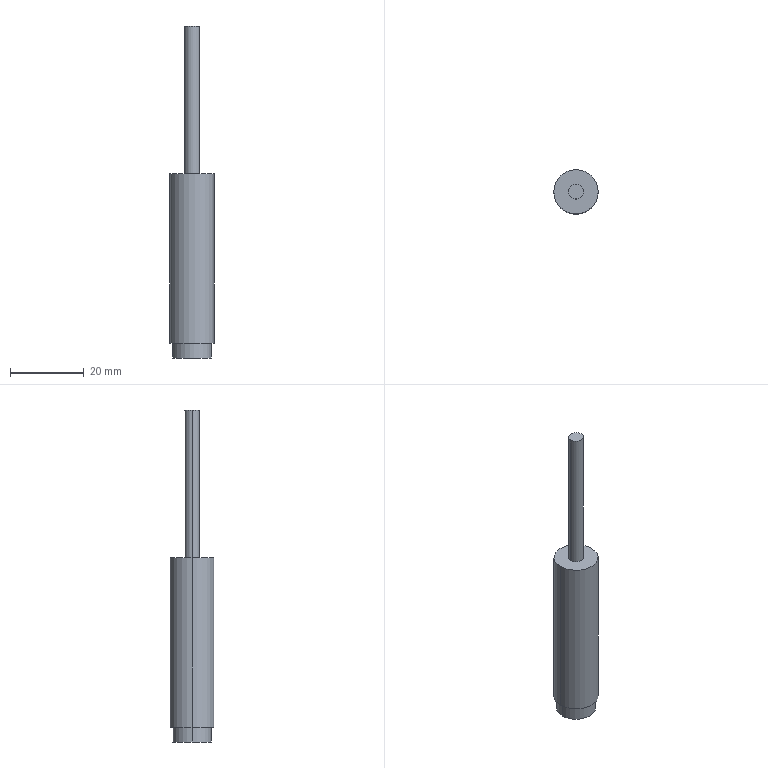Part | STEP file | PN_0035 (M12-4 proximity switch) | 1 solid | 10 faces | box 12 x 12 x 90 mm | volume 6055 mm3 | cylinder 6 | plane 4 | commonest cylinder face diameters 4 x2 10.55 x2 12 x2
STEP:
#1=CARTESIAN_POINT('',(0.,0.,0.));
#2=DIRECTION('',(0.,0.,1.));
#3=DIRECTION('',(1.,0.,0.));
#4=AXIS2_PLACEMENT_3D('',#1,#2,#3);
#5=CARTESIAN_POINT('',(2.,0.,90.));
#6=VERTEX_POINT('',#5);
#7=CARTESIAN_POINT('',(-2.,0.,90.));
#8=VERTEX_POINT('',#7);
#9=CARTESIAN_POINT('',(0.,0.,90.));
#10=DIRECTION('',(0.,0.,1.));
#11=DIRECTION('',(1.,0.,0.));
#12=AXIS2_PLACEMENT_3D('',#9,#10,#11);
#13=CIRCLE('',#12,2.);
#14=CARTESIAN_POINT('',(0.,0.,90.));
#15=DIRECTION('',(0.,0.,-1.));
#16=DIRECTION('',(-1.,0.,0.));
#17=AXIS2_PLACEMENT_3D('',#14,#15,#16);
#18=CYLINDRICAL_SURFACE('',#17,2.);
#19=CARTESIAN_POINT('',(3.142,0.));
#20=DIRECTION('',(-1.,0.));
#21=VECTOR('',#20,1.);
#22=LINE('',#19,#21);
#23=(GEOMETRIC_REPRESENTATION_CONTEXT(2)PARAMETRIC_REPRESENTATION_CONTEXT()REPRESENTATION_CONTEXT('',''));
#24=DEFINITIONAL_REPRESENTATION('',(#22),#23);
#25=PCURVE('',#18,#24);
#26=CARTESIAN_POINT('',(0.,0.,90.));
#27=DIRECTION('',(0.,0.,1.));
#28=DIRECTION('',(1.,0.,0.));
#29=AXIS2_PLACEMENT_3D('',#26,#27,#28);
#30=PLANE('',#29);
#31=CARTESIAN_POINT('',(0.,0.));
#32=DIRECTION('',(1.,0.));
#33=AXIS2_PLACEMENT_2D('',#31,#32);
#34=CIRCLE('',#33,2.);
#35=(GEOMETRIC_REPRESENTATION_CONTEXT(2)PARAMETRIC_REPRESENTATION_CONTEXT()REPRESENTATION_CONTEXT('',''));
#36=DEFINITIONAL_REPRESENTATION('',(#34),#35);
#37=PCURVE('',#30,#36);
#38=SURFACE_CURVE('',#13,(#25,#37),.PCURVE_S1.);
#39=EDGE_CURVE('',#6,#8,#38,.T.);
#40=ORIENTED_EDGE('',*,*,#39,.F.);
#41=CARTESIAN_POINT('',(2.,0.,50.));
#42=VERTEX_POINT('',#41);
#43=CARTESIAN_POINT('',(2.,0.,90.));
#44=DIRECTION('',(0.,0.,-1.));
#45=VECTOR('',#44,1.);
#46=LINE('',#43,#45);
#47=CARTESIAN_POINT('',(3.142,0.));
#48=DIRECTION('',(0.,1.));
#49=VECTOR('',#48,1.);
#50=LINE('',#47,#49);
#51=(GEOMETRIC_REPRESENTATION_CONTEXT(2)PARAMETRIC_REPRESENTATION_CONTEXT()REPRESENTATION_CONTEXT('',''));
#52=DEFINITIONAL_REPRESENTATION('',(#50),#51);
#53=PCURVE('',#18,#52);
#54=CARTESIAN_POINT('',(0.,0.,90.));
#55=DIRECTION('',(0.,0.,-1.));
#56=DIRECTION('',(-1.,0.,0.));
#57=AXIS2_PLACEMENT_3D('',#54,#55,#56);
#58=CYLINDRICAL_SURFACE('',#57,2.);
#59=CARTESIAN_POINT('',(3.142,0.));
#60=DIRECTION('',(0.,1.));
#61=VECTOR('',#60,1.);
#62=LINE('',#59,#61);
#63=(GEOMETRIC_REPRESENTATION_CONTEXT(2)PARAMETRIC_REPRESENTATION_CONTEXT()REPRESENTATION_CONTEXT('',''));
#64=DEFINITIONAL_REPRESENTATION('',(#62),#63);
#65=PCURVE('',#58,#64);
#66=SURFACE_CURVE('',#46,(#53,#65),.PCURVE_S1.);
#67=EDGE_CURVE('',#6,#42,#66,.T.);
#68=ORIENTED_EDGE('',*,*,#67,.T.);
#69=CARTESIAN_POINT('',(-2.,0.,50.));
#70=VERTEX_POINT('',#69);
#71=CARTESIAN_POINT('',(0.,0.,50.));
#72=DIRECTION('',(0.,0.,1.));
#73=DIRECTION('',(1.,0.,0.));
#74=AXIS2_PLACEMENT_3D('',#71,#72,#73);
#75=CIRCLE('',#74,2.);
#76=CARTESIAN_POINT('',(3.142,40.));
#77=DIRECTION('',(-1.,0.));
#78=VECTOR('',#77,1.);
#79=LINE('',#76,#78);
#80=(GEOMETRIC_REPRESENTATION_CONTEXT(2)PARAMETRIC_REPRESENTATION_CONTEXT()REPRESENTATION_CONTEXT('',''));
#81=DEFINITIONAL_REPRESENTATION('',(#79),#80);
#82=PCURVE('',#18,#81);
#83=CARTESIAN_POINT('',(0.,0.,50.));
#84=DIRECTION('',(0.,0.,1.));
#85=DIRECTION('',(1.,0.,0.));
#86=AXIS2_PLACEMENT_3D('',#83,#84,#85);
#87=PLANE('',#86);
#88=CARTESIAN_POINT('',(0.,0.));
#89=DIRECTION('',(1.,0.));
#90=AXIS2_PLACEMENT_2D('',#88,#89);
#91=CIRCLE('',#90,2.);
#92=(GEOMETRIC_REPRESENTATION_CONTEXT(2)PARAMETRIC_REPRESENTATION_CONTEXT()REPRESENTATION_CONTEXT('',''));
#93=DEFINITIONAL_REPRESENTATION('',(#91),#92);
#94=PCURVE('',#87,#93);
#95=SURFACE_CURVE('',#75,(#82,#94),.PCURVE_S1.);
#96=EDGE_CURVE('',#42,#70,#95,.T.);
#97=ORIENTED_EDGE('',*,*,#96,.T.);
#98=CARTESIAN_POINT('',(-2.,0.,90.));
#99=DIRECTION('',(0.,0.,-1.));
#100=VECTOR('',#99,1.);
#101=LINE('',#98,#100);
#102=CARTESIAN_POINT('',(0.,0.));
#103=DIRECTION('',(0.,1.));
#104=VECTOR('',#103,1.);
#105=LINE('',#102,#104);
#106=(GEOMETRIC_REPRESENTATION_CONTEXT(2)PARAMETRIC_REPRESENTATION_CONTEXT()REPRESENTATION_CONTEXT('',''));
#107=DEFINITIONAL_REPRESENTATION('',(#105),#106);
#108=PCURVE('',#18,#107);
#109=CARTESIAN_POINT('',(6.283,0.));
#110=DIRECTION('',(0.,1.));
#111=VECTOR('',#110,1.);
#112=LINE('',#109,#111);
#113=(GEOMETRIC_REPRESENTATION_CONTEXT(2)PARAMETRIC_REPRESENTATION_CONTEXT()REPRESENTATION_CONTEXT('',''));
#114=DEFINITIONAL_REPRESENTATION('',(#112),#113);
#115=PCURVE('',#58,#114);
#116=SURFACE_CURVE('',#101,(#108,#115),.PCURVE_S1.);
#117=EDGE_CURVE('',#8,#70,#116,.T.);
#118=ORIENTED_EDGE('',*,*,#117,.F.);
#119=EDGE_LOOP('',(#40,#68,#97,#118));
#120=FACE_BOUND('',#119,.T.);
#121=ADVANCED_FACE('',(#120),#18,.T.);
#122=CARTESIAN_POINT('',(6.,0.,50.));
#123=VERTEX_POINT('',#122);
#124=CARTESIAN_POINT('',(-6.,0.,50.));
#125=VERTEX_POINT('',#124);
#126=CARTESIAN_POINT('',(0.,0.,50.));
#127=DIRECTION('',(0.,0.,1.));
#128=DIRECTION('',(1.,0.,0.));
#129=AXIS2_PLACEMENT_3D('',#126,#127,#128);
#130=CIRCLE('',#129,6.);
#131=CARTESIAN_POINT('',(0.,0.,50.));
#132=DIRECTION('',(0.,0.,-1.));
#133=DIRECTION('',(-1.,0.,0.));
#134=AXIS2_PLACEMENT_3D('',#131,#132,#133);
#135=CYLINDRICAL_SURFACE('',#134,6.);
#136=CARTESIAN_POINT('',(3.142,0.));
#137=DIRECTION('',(-1.,0.));
#138=VECTOR('',#137,1.);
#139=LINE('',#136,#138);
#140=(GEOMETRIC_REPRESENTATION_CONTEXT(2)PARAMETRIC_REPRESENTATION_CONTEXT()REPRESENTATION_CONTEXT('',''));
#141=DEFINITIONAL_REPRESENTATION('',(#139),#140);
#142=PCURVE('',#135,#141);
#143=CARTESIAN_POINT('',(0.,0.));
#144=DIRECTION('',(1.,0.));
#145=AXIS2_PLACEMENT_2D('',#143,#144);
#146=CIRCLE('',#145,6.);
#147=(GEOMETRIC_REPRESENTATION_CONTEXT(2)PARAMETRIC_REPRESENTATION_CONTEXT()REPRESENTATION_CONTEXT('',''));
#148=DEFINITIONAL_REPRESENTATION('',(#146),#147);
#149=PCURVE('',#87,#148);
#150=SURFACE_CURVE('',#130,(#142,#149),.PCURVE_S1.);
#151=EDGE_CURVE('',#123,#125,#150,.T.);
#152=ORIENTED_EDGE('',*,*,#151,.F.);
#153=CARTESIAN_POINT('',(6.,0.,4.));
#154=VERTEX_POINT('',#153);
#155=CARTESIAN_POINT('',(6.,0.,50.));
#156=DIRECTION('',(0.,0.,-1.));
#157=VECTOR('',#156,1.);
#158=LINE('',#155,#157);
#159=CARTESIAN_POINT('',(3.142,0.));
#160=DIRECTION('',(0.,1.));
#161=VECTOR('',#160,1.);
#162=LINE('',#159,#161);
#163=(GEOMETRIC_REPRESENTATION_CONTEXT(2)PARAMETRIC_REPRESENTATION_CONTEXT()REPRESENTATION_CONTEXT('',''));
#164=DEFINITIONAL_REPRESENTATION('',(#162),#163);
#165=PCURVE('',#135,#164);
#166=CARTESIAN_POINT('',(0.,0.,50.));
#167=DIRECTION('',(0.,0.,-1.));
#168=DIRECTION('',(-1.,0.,0.));
#169=AXIS2_PLACEMENT_3D('',#166,#167,#168);
#170=CYLINDRICAL_SURFACE('',#169,6.);
#171=CARTESIAN_POINT('',(3.142,0.));
#172=DIRECTION('',(0.,1.));
#173=VECTOR('',#172,1.);
#174=LINE('',#171,#173);
#175=(GEOMETRIC_REPRESENTATION_CONTEXT(2)PARAMETRIC_REPRESENTATION_CONTEXT()REPRESENTATION_CONTEXT('',''));
#176=DEFINITIONAL_REPRESENTATION('',(#174),#175);
#177=PCURVE('',#170,#176);
#178=SURFACE_CURVE('',#158,(#165,#177),.PCURVE_S1.);
#179=EDGE_CURVE('',#123,#154,#178,.T.);
#180=ORIENTED_EDGE('',*,*,#179,.T.);
#181=CARTESIAN_POINT('',(-6.,0.,4.));
#182=VERTEX_POINT('',#181);
#183=CARTESIAN_POINT('',(0.,0.,4.));
#184=DIRECTION('',(0.,0.,1.));
#185=DIRECTION('',(1.,0.,0.));
#186=AXIS2_PLACEMENT_3D('',#183,#184,#185);
#187=CIRCLE('',#186,6.);
#188=CARTESIAN_POINT('',(3.142,46.));
#189=DIRECTION('',(-1.,0.));
#190=VECTOR('',#189,1.);
#191=LINE('',#188,#190);
#192=(GEOMETRIC_REPRESENTATION_CONTEXT(2)PARAMETRIC_REPRESENTATION_CONTEXT()REPRESENTATION_CONTEXT('',''));
#193=DEFINITIONAL_REPRESENTATION('',(#191),#192);
#194=PCURVE('',#135,#193);
#195=CARTESIAN_POINT('',(0.,0.,4.));
#196=DIRECTION('',(0.,0.,1.));
#197=DIRECTION('',(1.,0.,0.));
#198=AXIS2_PLACEMENT_3D('',#195,#196,#197);
#199=PLANE('',#198);
#200=CARTESIAN_POINT('',(0.,0.));
#201=DIRECTION('',(1.,0.));
#202=AXIS2_PLACEMENT_2D('',#200,#201);
#203=CIRCLE('',#202,6.);
#204=(GEOMETRIC_REPRESENTATION_CONTEXT(2)PARAMETRIC_REPRESENTATION_CONTEXT()REPRESENTATION_CONTEXT('',''));
#205=DEFINITIONAL_REPRESENTATION('',(#203),#204);
#206=PCURVE('',#199,#205);
#207=SURFACE_CURVE('',#187,(#194,#206),.PCURVE_S1.);
#208=EDGE_CURVE('',#154,#182,#207,.T.);
#209=ORIENTED_EDGE('',*,*,#208,.T.);
#210=CARTESIAN_POINT('',(-6.,0.,50.));
#211=DIRECTION('',(0.,0.,-1.));
#212=VECTOR('',#211,1.);
#213=LINE('',#210,#212);
#214=CARTESIAN_POINT('',(0.,0.));
#215=DIRECTION('',(0.,1.));
#216=VECTOR('',#215,1.);
#217=LINE('',#214,#216);
#218=(GEOMETRIC_REPRESENTATION_CONTEXT(2)PARAMETRIC_REPRESENTATION_CONTEXT()REPRESENTATION_CONTEXT('',''));
#219=DEFINITIONAL_REPRESENTATION('',(#217),#218);
#220=PCURVE('',#135,#219);
#221=CARTESIAN_POINT('',(6.283,0.));
#222=DIRECTION('',(0.,1.));
#223=VECTOR('',#222,1.);
#224=LINE('',#221,#223);
#225=(GEOMETRIC_REPRESENTATION_CONTEXT(2)PARAMETRIC_REPRESENTATION_CONTEXT()REPRESENTATION_CONTEXT('',''));
#226=DEFINITIONAL_REPRESENTATION('',(#224),#225);
#227=PCURVE('',#170,#226);
#228=SURFACE_CURVE('',#213,(#220,#227),.PCURVE_S1.);
#229=EDGE_CURVE('',#125,#182,#228,.T.);
#230=ORIENTED_EDGE('',*,*,#229,.F.);
#231=EDGE_LOOP('',(#152,#180,#209,#230));
#232=FACE_BOUND('',#231,.T.);
#233=ADVANCED_FACE('',(#232),#135,.T.);
#234=CARTESIAN_POINT('',(5.275,0.,4.));
#235=VERTEX_POINT('',#234);
#236=CARTESIAN_POINT('',(-5.275,0.,4.));
#237=VERTEX_POINT('',#236);
#238=CARTESIAN_POINT('',(0.,0.,4.));
#239=DIRECTION('',(0.,0.,1.));
#240=DIRECTION('',(1.,0.,0.));
#241=AXIS2_PLACEMENT_3D('',#238,#239,#240);
#242=CIRCLE('',#241,5.275);
#243=CARTESIAN_POINT('',(0.,0.,4.));
#244=DIRECTION('',(0.,0.,-1.));
#245=DIRECTION('',(-1.,0.,0.));
#246=AXIS2_PLACEMENT_3D('',#243,#244,#245);
#247=CYLINDRICAL_SURFACE('',#246,5.275);
#248=CARTESIAN_POINT('',(3.142,0.));
#249=DIRECTION('',(-1.,0.));
#250=VECTOR('',#249,1.);
#251=LINE('',#248,#250);
#252=(GEOMETRIC_REPRESENTATION_CONTEXT(2)PARAMETRIC_REPRESENTATION_CONTEXT()REPRESENTATION_CONTEXT('',''));
#253=DEFINITIONAL_REPRESENTATION('',(#251),#252);
#254=PCURVE('',#247,#253);
#255=CARTESIAN_POINT('',(0.,0.));
#256=DIRECTION('',(1.,0.));
#257=AXIS2_PLACEMENT_2D('',#255,#256);
#258=CIRCLE('',#257,5.275);
#259=(GEOMETRIC_REPRESENTATION_CONTEXT(2)PARAMETRIC_REPRESENTATION_CONTEXT()REPRESENTATION_CONTEXT('',''));
#260=DEFINITIONAL_REPRESENTATION('',(#258),#259);
#261=PCURVE('',#199,#260);
#262=SURFACE_CURVE('',#242,(#254,#261),.PCURVE_S1.);
#263=EDGE_CURVE('',#235,#237,#262,.T.);
#264=ORIENTED_EDGE('',*,*,#263,.F.);
#265=CARTESIAN_POINT('',(5.275,0.,0.));
#266=VERTEX_POINT('',#265);
#267=CARTESIAN_POINT('',(5.275,0.,4.));
#268=DIRECTION('',(0.,0.,-1.));
#269=VECTOR('',#268,1.);
#270=LINE('',#267,#269);
#271=CARTESIAN_POINT('',(3.142,0.));
#272=DIRECTION('',(0.,1.));
#273=VECTOR('',#272,1.);
#274=LINE('',#271,#273);
#275=(GEOMETRIC_REPRESENTATION_CONTEXT(2)PARAMETRIC_REPRESENTATION_CONTEXT()REPRESENTATION_CONTEXT('',''));
#276=DEFINITIONAL_REPRESENTATION('',(#274),#275);
#277=PCURVE('',#247,#276);
#278=CARTESIAN_POINT('',(0.,0.,4.));
#279=DIRECTION('',(0.,0.,-1.));
#280=DIRECTION('',(-1.,0.,0.));
#281=AXIS2_PLACEMENT_3D('',#278,#279,#280);
#282=CYLINDRICAL_SURFACE('',#281,5.275);
#283=CARTESIAN_POINT('',(3.142,0.));
#284=DIRECTION('',(0.,1.));
#285=VECTOR('',#284,1.);
#286=LINE('',#283,#285);
#287=(GEOMETRIC_REPRESENTATION_CONTEXT(2)PARAMETRIC_REPRESENTATION_CONTEXT()REPRESENTATION_CONTEXT('',''));
#288=DEFINITIONAL_REPRESENTATION('',(#286),#287);
#289=PCURVE('',#282,#288);
#290=SURFACE_CURVE('',#270,(#277,#289),.PCURVE_S1.);
#291=EDGE_CURVE('',#235,#266,#290,.T.);
#292=ORIENTED_EDGE('',*,*,#291,.T.);
#293=CARTESIAN_POINT('',(-5.275,0.,0.));
#294=VERTEX_POINT('',#293);
#295=CARTESIAN_POINT('',(0.,0.,0.));
#296=DIRECTION('',(0.,0.,1.));
#297=DIRECTION('',(1.,0.,0.));
#298=AXIS2_PLACEMENT_3D('',#295,#296,#297);
#299=CIRCLE('',#298,5.275);
#300=CARTESIAN_POINT('',(3.142,4.));
#301=DIRECTION('',(-1.,0.));
#302=VECTOR('',#301,1.);
#303=LINE('',#300,#302);
#304=(GEOMETRIC_REPRESENTATION_CONTEXT(2)PARAMETRIC_REPRESENTATION_CONTEXT()REPRESENTATION_CONTEXT('',''));
#305=DEFINITIONAL_REPRESENTATION('',(#303),#304);
#306=PCURVE('',#247,#305);
#307=CARTESIAN_POINT('',(0.,0.,0.));
#308=DIRECTION('',(0.,0.,1.));
#309=DIRECTION('',(1.,0.,0.));
#310=AXIS2_PLACEMENT_3D('',#307,#308,#309);
#311=PLANE('',#310);
#312=CARTESIAN_POINT('',(0.,0.));
#313=DIRECTION('',(1.,0.));
#314=AXIS2_PLACEMENT_2D('',#312,#313);
#315=CIRCLE('',#314,5.275);
#316=(GEOMETRIC_REPRESENTATION_CONTEXT(2)PARAMETRIC_REPRESENTATION_CONTEXT()REPRESENTATION_CONTEXT('',''));
#317=DEFINITIONAL_REPRESENTATION('',(#315),#316);
#318=PCURVE('',#311,#317);
#319=SURFACE_CURVE('',#299,(#306,#318),.PCURVE_S1.);
#320=EDGE_CURVE('',#266,#294,#319,.T.);
#321=ORIENTED_EDGE('',*,*,#320,.T.);
#322=CARTESIAN_POINT('',(-5.275,0.,4.));
#323=DIRECTION('',(0.,0.,-1.));
#324=VECTOR('',#323,1.);
#325=LINE('',#322,#324);
#326=CARTESIAN_POINT('',(0.,0.));
#327=DIRECTION('',(0.,1.));
#328=VECTOR('',#327,1.);
#329=LINE('',#326,#328);
#330=(GEOMETRIC_REPRESENTATION_CONTEXT(2)PARAMETRIC_REPRESENTATION_CONTEXT()REPRESENTATION_CONTEXT('',''));
#331=DEFINITIONAL_REPRESENTATION('',(#329),#330);
#332=PCURVE('',#247,#331);
#333=CARTESIAN_POINT('',(6.283,0.));
#334=DIRECTION('',(0.,1.));
#335=VECTOR('',#334,1.);
#336=LINE('',#333,#335);
#337=(GEOMETRIC_REPRESENTATION_CONTEXT(2)PARAMETRIC_REPRESENTATION_CONTEXT()REPRESENTATION_CONTEXT('',''));
#338=DEFINITIONAL_REPRESENTATION('',(#336),#337);
#339=PCURVE('',#282,#338);
#340=SURFACE_CURVE('',#325,(#332,#339),.PCURVE_S1.);
#341=EDGE_CURVE('',#237,#294,#340,.T.);
#342=ORIENTED_EDGE('',*,*,#341,.F.);
#343=EDGE_LOOP('',(#264,#292,#321,#342));
#344=FACE_BOUND('',#343,.T.);
#345=ADVANCED_FACE('',(#344),#247,.T.);
#346=CARTESIAN_POINT('',(0.,0.,50.));
#347=DIRECTION('',(0.,0.,1.));
#348=DIRECTION('',(1.,0.,0.));
#349=AXIS2_PLACEMENT_3D('',#346,#347,#348);
#350=CIRCLE('',#349,6.);
#351=CARTESIAN_POINT('',(0.,0.));
#352=DIRECTION('',(1.,0.));
#353=AXIS2_PLACEMENT_2D('',#351,#352);
#354=CIRCLE('',#353,6.);
#355=(GEOMETRIC_REPRESENTATION_CONTEXT(2)PARAMETRIC_REPRESENTATION_CONTEXT()REPRESENTATION_CONTEXT('',''));
#356=DEFINITIONAL_REPRESENTATION('',(#354),#355);
#357=PCURVE('',#87,#356);
#358=CARTESIAN_POINT('',(9.425,0.));
#359=DIRECTION('',(-1.,0.));
#360=VECTOR('',#359,1.);
#361=LINE('',#358,#360);
#362=(GEOMETRIC_REPRESENTATION_CONTEXT(2)PARAMETRIC_REPRESENTATION_CONTEXT()REPRESENTATION_CONTEXT('',''));
#363=DEFINITIONAL_REPRESENTATION('',(#361),#362);
#364=PCURVE('',#170,#363);
#365=SURFACE_CURVE('',#350,(#357,#364),.PCURVE_S1.);
#366=EDGE_CURVE('',#125,#123,#365,.T.);
#367=ORIENTED_EDGE('',*,*,#366,.T.);
#368=ORIENTED_EDGE('',*,*,#151,.T.);
#369=EDGE_LOOP('',(#367,#368));
#370=FACE_BOUND('',#369,.T.);
#371=CARTESIAN_POINT('',(0.,0.,50.));
#372=DIRECTION('',(0.,0.,1.));
#373=DIRECTION('',(1.,0.,0.));
#374=AXIS2_PLACEMENT_3D('',#371,#372,#373);
#375=CIRCLE('',#374,2.);
#376=CARTESIAN_POINT('',(0.,0.));
#377=DIRECTION('',(1.,0.));
#378=AXIS2_PLACEMENT_2D('',#376,#377);
#379=CIRCLE('',#378,2.);
#380=(GEOMETRIC_REPRESENTATION_CONTEXT(2)PARAMETRIC_REPRESENTATION_CONTEXT()REPRESENTATION_CONTEXT('',''));
#381=DEFINITIONAL_REPRESENTATION('',(#379),#380);
#382=PCURVE('',#87,#381);
#383=CARTESIAN_POINT('',(9.425,40.));
#384=DIRECTION('',(-1.,0.));
#385=VECTOR('',#384,1.);
#386=LINE('',#383,#385);
#387=(GEOMETRIC_REPRESENTATION_CONTEXT(2)PARAMETRIC_REPRESENTATION_CONTEXT()REPRESENTATION_CONTEXT('',''));
#388=DEFINITIONAL_REPRESENTATION('',(#386),#387);
#389=PCURVE('',#58,#388);
#390=SURFACE_CURVE('',#375,(#382,#389),.PCURVE_S1.);
#391=EDGE_CURVE('',#70,#42,#390,.T.);
#392=ORIENTED_EDGE('',*,*,#391,.F.);
#393=ORIENTED_EDGE('',*,*,#96,.F.);
#394=EDGE_LOOP('',(#392,#393));
#395=FACE_BOUND('',#394,.T.);
#396=ADVANCED_FACE('',(#370,#395),#87,.T.);
#397=ORIENTED_EDGE('',*,*,#291,.F.);
#398=CARTESIAN_POINT('',(0.,0.,4.));
#399=DIRECTION('',(0.,0.,1.));
#400=DIRECTION('',(1.,0.,0.));
#401=AXIS2_PLACEMENT_3D('',#398,#399,#400);
#402=CIRCLE('',#401,5.275);
#403=CARTESIAN_POINT('',(9.425,0.));
#404=DIRECTION('',(-1.,0.));
#405=VECTOR('',#404,1.);
#406=LINE('',#403,#405);
#407=(GEOMETRIC_REPRESENTATION_CONTEXT(2)PARAMETRIC_REPRESENTATION_CONTEXT()REPRESENTATION_CONTEXT('',''));
#408=DEFINITIONAL_REPRESENTATION('',(#406),#407);
#409=PCURVE('',#282,#408);
#410=CARTESIAN_POINT('',(0.,0.));
#411=DIRECTION('',(1.,0.));
#412=AXIS2_PLACEMENT_2D('',#410,#411);
#413=CIRCLE('',#412,5.275);
#414=(GEOMETRIC_REPRESENTATION_CONTEXT(2)PARAMETRIC_REPRESENTATION_CONTEXT()REPRESENTATION_CONTEXT('',''));
#415=DEFINITIONAL_REPRESENTATION('',(#413),#414);
#416=PCURVE('',#199,#415);
#417=SURFACE_CURVE('',#402,(#409,#416),.PCURVE_S1.);
#418=EDGE_CURVE('',#237,#235,#417,.T.);
#419=ORIENTED_EDGE('',*,*,#418,.F.);
#420=ORIENTED_EDGE('',*,*,#341,.T.);
#421=CARTESIAN_POINT('',(0.,0.,0.));
#422=DIRECTION('',(0.,0.,1.));
#423=DIRECTION('',(1.,0.,0.));
#424=AXIS2_PLACEMENT_3D('',#421,#422,#423);
#425=CIRCLE('',#424,5.275);
#426=CARTESIAN_POINT('',(9.425,4.));
#427=DIRECTION('',(-1.,0.));
#428=VECTOR('',#427,1.);
#429=LINE('',#426,#428);
#430=(GEOMETRIC_REPRESENTATION_CONTEXT(2)PARAMETRIC_REPRESENTATION_CONTEXT()REPRESENTATION_CONTEXT('',''));
#431=DEFINITIONAL_REPRESENTATION('',(#429),#430);
#432=PCURVE('',#282,#431);
#433=CARTESIAN_POINT('',(0.,0.));
#434=DIRECTION('',(1.,0.));
#435=AXIS2_PLACEMENT_2D('',#433,#434);
#436=CIRCLE('',#435,5.275);
#437=(GEOMETRIC_REPRESENTATION_CONTEXT(2)PARAMETRIC_REPRESENTATION_CONTEXT()REPRESENTATION_CONTEXT('',''));
#438=DEFINITIONAL_REPRESENTATION('',(#436),#437);
#439=PCURVE('',#311,#438);
#440=SURFACE_CURVE('',#425,(#432,#439),.PCURVE_S1.);
#441=EDGE_CURVE('',#294,#266,#440,.T.);
#442=ORIENTED_EDGE('',*,*,#441,.T.);
#443=EDGE_LOOP('',(#397,#419,#420,#442));
#444=FACE_BOUND('',#443,.T.);
#445=ADVANCED_FACE('',(#444),#282,.T.);
#446=ORIENTED_EDGE('',*,*,#441,.F.);
#447=ORIENTED_EDGE('',*,*,#320,.F.);
#448=EDGE_LOOP('',(#446,#447));
#449=FACE_BOUND('',#448,.T.);
#450=ADVANCED_FACE('',(#449),#311,.F.);
#451=CARTESIAN_POINT('',(0.,0.,4.));
#452=DIRECTION('',(0.,0.,1.));
#453=DIRECTION('',(1.,0.,0.));
#454=AXIS2_PLACEMENT_3D('',#451,#452,#453);
#455=CIRCLE('',#454,6.);
#456=CARTESIAN_POINT('',(0.,0.));
#457=DIRECTION('',(1.,0.));
#458=AXIS2_PLACEMENT_2D('',#456,#457);
#459=CIRCLE('',#458,6.);
#460=(GEOMETRIC_REPRESENTATION_CONTEXT(2)PARAMETRIC_REPRESENTATION_CONTEXT()REPRESENTATION_CONTEXT('',''));
#461=DEFINITIONAL_REPRESENTATION('',(#459),#460);
#462=PCURVE('',#199,#461);
#463=CARTESIAN_POINT('',(9.425,46.));
#464=DIRECTION('',(-1.,0.));
#465=VECTOR('',#464,1.);
#466=LINE('',#463,#465);
#467=(GEOMETRIC_REPRESENTATION_CONTEXT(2)PARAMETRIC_REPRESENTATION_CONTEXT()REPRESENTATION_CONTEXT('',''));
#468=DEFINITIONAL_REPRESENTATION('',(#466),#467);
#469=PCURVE('',#170,#468);
#470=SURFACE_CURVE('',#455,(#462,#469),.PCURVE_S1.);
#471=EDGE_CURVE('',#182,#154,#470,.T.);
#472=ORIENTED_EDGE('',*,*,#471,.F.);
#473=ORIENTED_EDGE('',*,*,#208,.F.);
#474=EDGE_LOOP('',(#472,#473));
#475=FACE_BOUND('',#474,.T.);
#476=ORIENTED_EDGE('',*,*,#418,.T.);
#477=ORIENTED_EDGE('',*,*,#263,.T.);
#478=EDGE_LOOP('',(#476,#477));
#479=FACE_BOUND('',#478,.T.);
#480=ADVANCED_FACE('',(#475,#479),#199,.F.);
#481=ORIENTED_EDGE('',*,*,#179,.F.);
#482=ORIENTED_EDGE('',*,*,#366,.F.);
#483=ORIENTED_EDGE('',*,*,#229,.T.);
#484=ORIENTED_EDGE('',*,*,#471,.T.);
#485=EDGE_LOOP('',(#481,#482,#483,#484));
#486=FACE_BOUND('',#485,.T.);
#487=ADVANCED_FACE('',(#486),#170,.T.);
#488=ORIENTED_EDGE('',*,*,#67,.F.);
#489=CARTESIAN_POINT('',(0.,0.,90.));
#490=DIRECTION('',(0.,0.,1.));
#491=DIRECTION('',(1.,0.,0.));
#492=AXIS2_PLACEMENT_3D('',#489,#490,#491);
#493=CIRCLE('',#492,2.);
#494=CARTESIAN_POINT('',(9.425,0.));
#495=DIRECTION('',(-1.,0.));
#496=VECTOR('',#495,1.);
#497=LINE('',#494,#496);
#498=(GEOMETRIC_REPRESENTATION_CONTEXT(2)PARAMETRIC_REPRESENTATION_CONTEXT()REPRESENTATION_CONTEXT('',''));
#499=DEFINITIONAL_REPRESENTATION('',(#497),#498);
#500=PCURVE('',#58,#499);
#501=CARTESIAN_POINT('',(0.,0.));
#502=DIRECTION('',(1.,0.));
#503=AXIS2_PLACEMENT_2D('',#501,#502);
#504=CIRCLE('',#503,2.);
#505=(GEOMETRIC_REPRESENTATION_CONTEXT(2)PARAMETRIC_REPRESENTATION_CONTEXT()REPRESENTATION_CONTEXT('',''));
#506=DEFINITIONAL_REPRESENTATION('',(#504),#505);
#507=PCURVE('',#30,#506);
#508=SURFACE_CURVE('',#493,(#500,#507),.PCURVE_S1.);
#509=EDGE_CURVE('',#8,#6,#508,.T.);
#510=ORIENTED_EDGE('',*,*,#509,.F.);
#511=ORIENTED_EDGE('',*,*,#117,.T.);
#512=ORIENTED_EDGE('',*,*,#391,.T.);
#513=EDGE_LOOP('',(#488,#510,#511,#512));
#514=FACE_BOUND('',#513,.T.);
#515=ADVANCED_FACE('',(#514),#58,.T.);
#516=ORIENTED_EDGE('',*,*,#509,.T.);
#517=ORIENTED_EDGE('',*,*,#39,.T.);
#518=EDGE_LOOP('',(#516,#517));
#519=FACE_BOUND('',#518,.T.);
#520=ADVANCED_FACE('',(#519),#30,.T.);
#521=CLOSED_SHELL('',(#121,#233,#345,#396,#445,#450,#480,#487,#515,#520));
#522=MANIFOLD_SOLID_BREP('',#521);
#523=(LENGTH_UNIT()NAMED_UNIT(*)SI_UNIT(.MILLI.,.METRE.));
#524=UNCERTAINTY_MEASURE_WITH_UNIT(LENGTH_MEASURE(0.0000001),#523,'','');
#525=(NAMED_UNIT(*)PLANE_ANGLE_UNIT()SI_UNIT($,.RADIAN.));
#526=(NAMED_UNIT(*)SI_UNIT($,.STERADIAN.)SOLID_ANGLE_UNIT());
#527=(GEOMETRIC_REPRESENTATION_CONTEXT(3)GLOBAL_UNCERTAINTY_ASSIGNED_CONTEXT((#524))GLOBAL_UNIT_ASSIGNED_CONTEXT((#523,#525,#526))REPRESENTATION_CONTEXT('',''));
#528=ADVANCED_BREP_SHAPE_REPRESENTATION('',(#4,#522),#527);